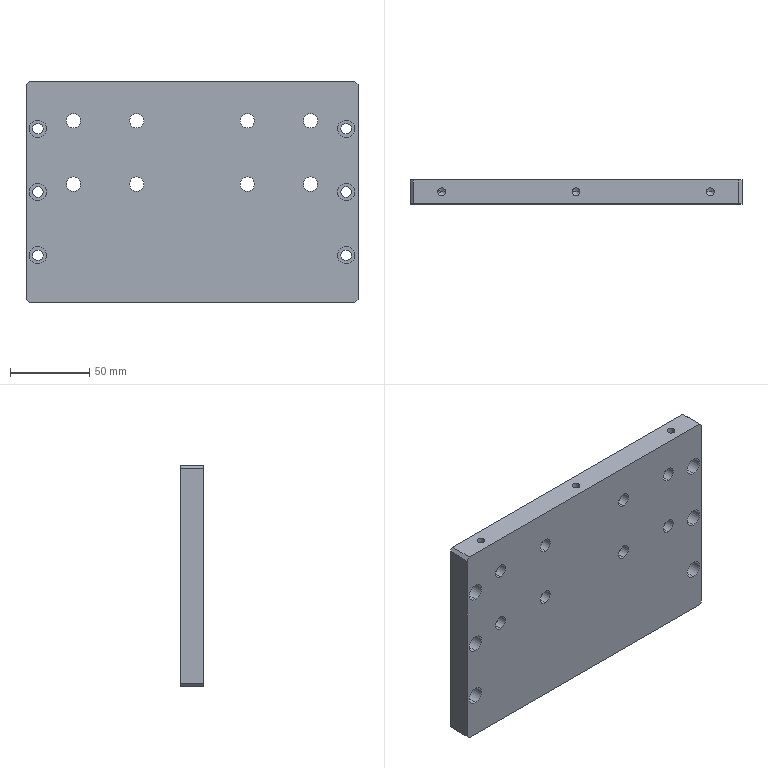Part | SolidWorks | features BaseBody 1 | 1 solid | 92 faces | box 210 x 15 x 140 mm | volume 418074 mm3 | cylinder 62 | plane 24 | cone 6 | commonest cylinder face diameters 9 x16 15 x16 6.6 x12 11 x12 5 x6